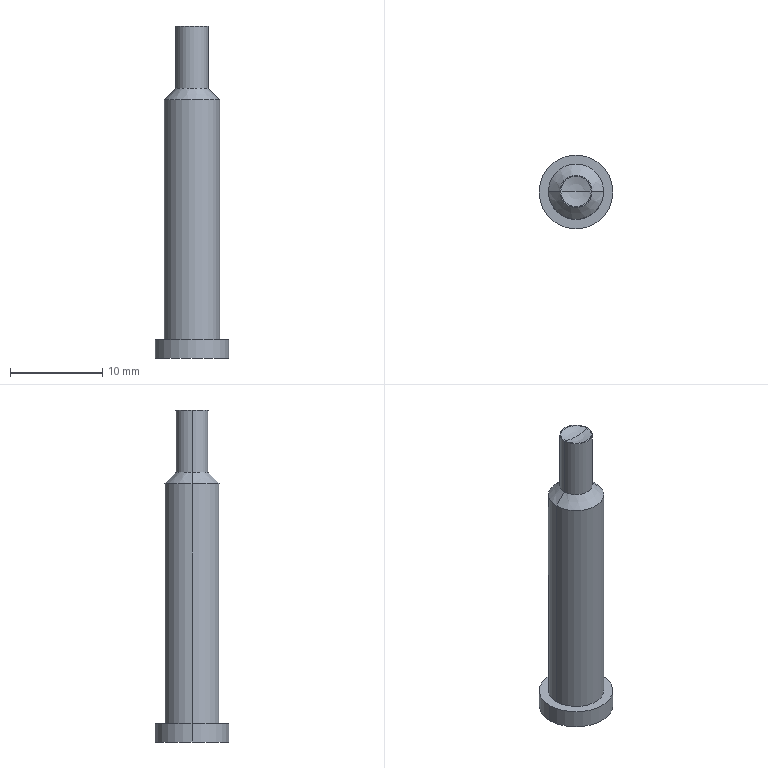Part | STEP file | Hot-melt nozzle | 1 solid | 13 faces | box 8 x 8 x 36 mm | volume 921.971 mm3 | cylinder 6 | plane 3 | cone 2 | sphere 2 | commonest cylinder face diameters 3.5 x2 6 x2 8 x2
STEP:
#1=CARTESIAN_POINT('',(0.,0.,0.));
#2=DIRECTION('',(0.,0.,1.));
#3=DIRECTION('',(1.,0.,0.));
#4=AXIS2_PLACEMENT_3D('',#1,#2,#3);
#5=CARTESIAN_POINT('',(139.55,-164.6,-40.7));
#6=VERTEX_POINT('',#5);
#7=CARTESIAN_POINT('',(147.55,-164.6,-40.7));
#8=VERTEX_POINT('',#7);
#9=CARTESIAN_POINT('',(143.55,-164.6,-40.7));
#10=DIRECTION('',(0.,0.,-1.));
#11=DIRECTION('',(-1.,0.,0.));
#12=AXIS2_PLACEMENT_3D('',#9,#10,#11);
#13=CIRCLE('',#12,4.);
#14=CARTESIAN_POINT('',(0.,0.,-40.7));
#15=DIRECTION('',(0.,0.,-1.));
#16=DIRECTION('',(-1.,0.,0.));
#17=AXIS2_PLACEMENT_3D('',#14,#15,#16);
#18=PLANE('',#17);
#19=CARTESIAN_POINT('',(-143.55,-164.6));
#20=DIRECTION('',(1.,0.));
#21=AXIS2_PLACEMENT_2D('',#19,#20);
#22=CIRCLE('',#21,4.);
#23=(GEOMETRIC_REPRESENTATION_CONTEXT(2)PARAMETRIC_REPRESENTATION_CONTEXT()REPRESENTATION_CONTEXT('',''));
#24=DEFINITIONAL_REPRESENTATION('',(#22),#23);
#25=PCURVE('',#18,#24);
#26=CARTESIAN_POINT('',(143.55,-164.6,-40.7));
#27=DIRECTION('',(0.,0.,-1.));
#28=DIRECTION('',(-1.,0.,0.));
#29=AXIS2_PLACEMENT_3D('',#26,#27,#28);
#30=CYLINDRICAL_SURFACE('',#29,4.);
#31=CARTESIAN_POINT('',(0.,0.));
#32=DIRECTION('',(1.,0.));
#33=VECTOR('',#32,1.);
#34=LINE('',#31,#33);
#35=(GEOMETRIC_REPRESENTATION_CONTEXT(2)PARAMETRIC_REPRESENTATION_CONTEXT()REPRESENTATION_CONTEXT('',''));
#36=DEFINITIONAL_REPRESENTATION('',(#34),#35);
#37=PCURVE('',#30,#36);
#38=SURFACE_CURVE('',#13,(#25,#37),.PCURVE_S1.);
#39=EDGE_CURVE('',#6,#8,#38,.T.);
#40=ORIENTED_EDGE('',*,*,#39,.F.);
#41=CARTESIAN_POINT('',(143.55,-164.6,-40.7));
#42=DIRECTION('',(0.,0.,-1.));
#43=DIRECTION('',(1.,0.,0.));
#44=AXIS2_PLACEMENT_3D('',#41,#42,#43);
#45=CIRCLE('',#44,4.);
#46=CARTESIAN_POINT('',(-143.55,-164.6));
#47=DIRECTION('',(-1.,0.));
#48=AXIS2_PLACEMENT_2D('',#46,#47);
#49=CIRCLE('',#48,4.);
#50=(GEOMETRIC_REPRESENTATION_CONTEXT(2)PARAMETRIC_REPRESENTATION_CONTEXT()REPRESENTATION_CONTEXT('',''));
#51=DEFINITIONAL_REPRESENTATION('',(#49),#50);
#52=PCURVE('',#18,#51);
#53=CARTESIAN_POINT('',(143.55,-164.6,-40.7));
#54=DIRECTION('',(0.,0.,-1.));
#55=DIRECTION('',(-1.,0.,0.));
#56=AXIS2_PLACEMENT_3D('',#53,#54,#55);
#57=CYLINDRICAL_SURFACE('',#56,4.);
#58=CARTESIAN_POINT('',(3.142,0.));
#59=DIRECTION('',(1.,0.));
#60=VECTOR('',#59,1.);
#61=LINE('',#58,#60);
#62=(GEOMETRIC_REPRESENTATION_CONTEXT(2)PARAMETRIC_REPRESENTATION_CONTEXT()REPRESENTATION_CONTEXT('',''));
#63=DEFINITIONAL_REPRESENTATION('',(#61),#62);
#64=PCURVE('',#57,#63);
#65=SURFACE_CURVE('',#45,(#52,#64),.PCURVE_S1.);
#66=EDGE_CURVE('',#8,#6,#65,.T.);
#67=ORIENTED_EDGE('',*,*,#66,.F.);
#68=EDGE_LOOP('',(#40,#67));
#69=FACE_BOUND('',#68,.F.);
#70=ADVANCED_FACE('',(#69),#18,.T.);
#71=CARTESIAN_POINT('',(139.55,-164.6,-38.7));
#72=VERTEX_POINT('',#71);
#73=CARTESIAN_POINT('',(139.55,-164.6,-40.7));
#74=DIRECTION('',(0.,0.,1.));
#75=VECTOR('',#74,1.);
#76=LINE('',#73,#75);
#77=CARTESIAN_POINT('',(0.,0.));
#78=DIRECTION('',(0.,-1.));
#79=VECTOR('',#78,1.);
#80=LINE('',#77,#79);
#81=(GEOMETRIC_REPRESENTATION_CONTEXT(2)PARAMETRIC_REPRESENTATION_CONTEXT()REPRESENTATION_CONTEXT('',''));
#82=DEFINITIONAL_REPRESENTATION('',(#80),#81);
#83=PCURVE('',#30,#82);
#84=CARTESIAN_POINT('',(6.283,0.));
#85=DIRECTION('',(0.,-1.));
#86=VECTOR('',#85,1.);
#87=LINE('',#84,#86);
#88=(GEOMETRIC_REPRESENTATION_CONTEXT(2)PARAMETRIC_REPRESENTATION_CONTEXT()REPRESENTATION_CONTEXT('',''));
#89=DEFINITIONAL_REPRESENTATION('',(#87),#88);
#90=PCURVE('',#57,#89);
#91=SURFACE_CURVE('',#76,(#83,#90),.PCURVE_S1.);
#92=EDGE_CURVE('',#6,#72,#91,.T.);
#93=ORIENTED_EDGE('',*,*,#92,.T.);
#94=CARTESIAN_POINT('',(147.55,-164.6,-38.7));
#95=VERTEX_POINT('',#94);
#96=CARTESIAN_POINT('',(143.55,-164.6,-38.7));
#97=DIRECTION('',(0.,0.,-1.));
#98=DIRECTION('',(-1.,0.,0.));
#99=AXIS2_PLACEMENT_3D('',#96,#97,#98);
#100=CIRCLE('',#99,4.);
#101=CARTESIAN_POINT('',(0.,-2.));
#102=DIRECTION('',(1.,0.));
#103=VECTOR('',#102,1.);
#104=LINE('',#101,#103);
#105=(GEOMETRIC_REPRESENTATION_CONTEXT(2)PARAMETRIC_REPRESENTATION_CONTEXT()REPRESENTATION_CONTEXT('',''));
#106=DEFINITIONAL_REPRESENTATION('',(#104),#105);
#107=PCURVE('',#30,#106);
#108=CARTESIAN_POINT('',(0.,0.,-38.7));
#109=DIRECTION('',(0.,0.,-1.));
#110=DIRECTION('',(-1.,0.,0.));
#111=AXIS2_PLACEMENT_3D('',#108,#109,#110);
#112=PLANE('',#111);
#113=CARTESIAN_POINT('',(-143.55,-164.6));
#114=DIRECTION('',(1.,0.));
#115=AXIS2_PLACEMENT_2D('',#113,#114);
#116=CIRCLE('',#115,4.);
#117=(GEOMETRIC_REPRESENTATION_CONTEXT(2)PARAMETRIC_REPRESENTATION_CONTEXT()REPRESENTATION_CONTEXT('',''));
#118=DEFINITIONAL_REPRESENTATION('',(#116),#117);
#119=PCURVE('',#112,#118);
#120=SURFACE_CURVE('',#100,(#107,#119),.PCURVE_S1.);
#121=EDGE_CURVE('',#72,#95,#120,.T.);
#122=ORIENTED_EDGE('',*,*,#121,.T.);
#123=CARTESIAN_POINT('',(147.55,-164.6,-40.7));
#124=DIRECTION('',(0.,0.,1.));
#125=VECTOR('',#124,1.);
#126=LINE('',#123,#125);
#127=CARTESIAN_POINT('',(3.142,0.));
#128=DIRECTION('',(0.,-1.));
#129=VECTOR('',#128,1.);
#130=LINE('',#127,#129);
#131=(GEOMETRIC_REPRESENTATION_CONTEXT(2)PARAMETRIC_REPRESENTATION_CONTEXT()REPRESENTATION_CONTEXT('',''));
#132=DEFINITIONAL_REPRESENTATION('',(#130),#131);
#133=PCURVE('',#30,#132);
#134=CARTESIAN_POINT('',(3.142,0.));
#135=DIRECTION('',(0.,-1.));
#136=VECTOR('',#135,1.);
#137=LINE('',#134,#136);
#138=(GEOMETRIC_REPRESENTATION_CONTEXT(2)PARAMETRIC_REPRESENTATION_CONTEXT()REPRESENTATION_CONTEXT('',''));
#139=DEFINITIONAL_REPRESENTATION('',(#137),#138);
#140=PCURVE('',#57,#139);
#141=SURFACE_CURVE('',#126,(#133,#140),.PCURVE_S1.);
#142=EDGE_CURVE('',#8,#95,#141,.T.);
#143=ORIENTED_EDGE('',*,*,#142,.F.);
#144=ORIENTED_EDGE('',*,*,#39,.F.);
#145=EDGE_LOOP('',(#93,#122,#143,#144));
#146=FACE_BOUND('',#145,.T.);
#147=ADVANCED_FACE('',(#146),#30,.T.);
#148=ORIENTED_EDGE('',*,*,#142,.T.);
#149=CARTESIAN_POINT('',(143.55,-164.6,-38.7));
#150=DIRECTION('',(0.,0.,-1.));
#151=DIRECTION('',(1.,0.,0.));
#152=AXIS2_PLACEMENT_3D('',#149,#150,#151);
#153=CIRCLE('',#152,4.);
#154=CARTESIAN_POINT('',(3.142,-2.));
#155=DIRECTION('',(1.,0.));
#156=VECTOR('',#155,1.);
#157=LINE('',#154,#156);
#158=(GEOMETRIC_REPRESENTATION_CONTEXT(2)PARAMETRIC_REPRESENTATION_CONTEXT()REPRESENTATION_CONTEXT('',''));
#159=DEFINITIONAL_REPRESENTATION('',(#157),#158);
#160=PCURVE('',#57,#159);
#161=CARTESIAN_POINT('',(-143.55,-164.6));
#162=DIRECTION('',(-1.,0.));
#163=AXIS2_PLACEMENT_2D('',#161,#162);
#164=CIRCLE('',#163,4.);
#165=(GEOMETRIC_REPRESENTATION_CONTEXT(2)PARAMETRIC_REPRESENTATION_CONTEXT()REPRESENTATION_CONTEXT('',''));
#166=DEFINITIONAL_REPRESENTATION('',(#164),#165);
#167=PCURVE('',#112,#166);
#168=SURFACE_CURVE('',#153,(#160,#167),.PCURVE_S1.);
#169=EDGE_CURVE('',#95,#72,#168,.T.);
#170=ORIENTED_EDGE('',*,*,#169,.T.);
#171=ORIENTED_EDGE('',*,*,#92,.F.);
#172=ORIENTED_EDGE('',*,*,#66,.F.);
#173=EDGE_LOOP('',(#148,#170,#171,#172));
#174=FACE_BOUND('',#173,.T.);
#175=ADVANCED_FACE('',(#174),#57,.T.);
#176=ORIENTED_EDGE('',*,*,#121,.T.);
#177=ORIENTED_EDGE('',*,*,#169,.T.);
#178=EDGE_LOOP('',(#176,#177));
#179=FACE_BOUND('',#178,.F.);
#180=CARTESIAN_POINT('',(140.55,-164.6,-38.7));
#181=VERTEX_POINT('',#180);
#182=CARTESIAN_POINT('',(146.55,-164.6,-38.7));
#183=VERTEX_POINT('',#182);
#184=CARTESIAN_POINT('',(143.55,-164.6,-38.7));
#185=DIRECTION('',(0.,0.,-1.));
#186=DIRECTION('',(-1.,0.,0.));
#187=AXIS2_PLACEMENT_3D('',#184,#185,#186);
#188=CIRCLE('',#187,3.);
#189=CARTESIAN_POINT('',(-143.55,-164.6));
#190=DIRECTION('',(1.,0.));
#191=AXIS2_PLACEMENT_2D('',#189,#190);
#192=CIRCLE('',#191,3.);
#193=(GEOMETRIC_REPRESENTATION_CONTEXT(2)PARAMETRIC_REPRESENTATION_CONTEXT()REPRESENTATION_CONTEXT('',''));
#194=DEFINITIONAL_REPRESENTATION('',(#192),#193);
#195=PCURVE('',#112,#194);
#196=CARTESIAN_POINT('',(143.55,-164.6,-40.7));
#197=DIRECTION('',(0.,0.,-1.));
#198=DIRECTION('',(-1.,0.,0.));
#199=AXIS2_PLACEMENT_3D('',#196,#197,#198);
#200=CYLINDRICAL_SURFACE('',#199,3.);
#201=CARTESIAN_POINT('',(0.,-2.));
#202=DIRECTION('',(1.,0.));
#203=VECTOR('',#202,1.);
#204=LINE('',#201,#203);
#205=(GEOMETRIC_REPRESENTATION_CONTEXT(2)PARAMETRIC_REPRESENTATION_CONTEXT()REPRESENTATION_CONTEXT('',''));
#206=DEFINITIONAL_REPRESENTATION('',(#204),#205);
#207=PCURVE('',#200,#206);
#208=SURFACE_CURVE('',#188,(#195,#207),.PCURVE_S1.);
#209=EDGE_CURVE('',#181,#183,#208,.T.);
#210=ORIENTED_EDGE('',*,*,#209,.F.);
#211=CARTESIAN_POINT('',(143.55,-164.6,-38.7));
#212=DIRECTION('',(0.,0.,-1.));
#213=DIRECTION('',(1.,0.,0.));
#214=AXIS2_PLACEMENT_3D('',#211,#212,#213);
#215=CIRCLE('',#214,3.);
#216=CARTESIAN_POINT('',(-143.55,-164.6));
#217=DIRECTION('',(-1.,0.));
#218=AXIS2_PLACEMENT_2D('',#216,#217);
#219=CIRCLE('',#218,3.);
#220=(GEOMETRIC_REPRESENTATION_CONTEXT(2)PARAMETRIC_REPRESENTATION_CONTEXT()REPRESENTATION_CONTEXT('',''));
#221=DEFINITIONAL_REPRESENTATION('',(#219),#220);
#222=PCURVE('',#112,#221);
#223=CARTESIAN_POINT('',(143.55,-164.6,-40.7));
#224=DIRECTION('',(0.,0.,-1.));
#225=DIRECTION('',(-1.,0.,0.));
#226=AXIS2_PLACEMENT_3D('',#223,#224,#225);
#227=CYLINDRICAL_SURFACE('',#226,3.);
#228=CARTESIAN_POINT('',(3.142,-2.));
#229=DIRECTION('',(1.,0.));
#230=VECTOR('',#229,1.);
#231=LINE('',#228,#230);
#232=(GEOMETRIC_REPRESENTATION_CONTEXT(2)PARAMETRIC_REPRESENTATION_CONTEXT()REPRESENTATION_CONTEXT('',''));
#233=DEFINITIONAL_REPRESENTATION('',(#231),#232);
#234=PCURVE('',#227,#233);
#235=SURFACE_CURVE('',#215,(#222,#234),.PCURVE_S1.);
#236=EDGE_CURVE('',#183,#181,#235,.T.);
#237=ORIENTED_EDGE('',*,*,#236,.F.);
#238=EDGE_LOOP('',(#210,#237));
#239=FACE_BOUND('',#238,.F.);
#240=ADVANCED_FACE('',(#179,#239),#112,.F.);
#241=CARTESIAN_POINT('',(146.55,-164.6,-12.7));
#242=VERTEX_POINT('',#241);
#243=CARTESIAN_POINT('',(146.55,-164.6,-38.7));
#244=DIRECTION('',(-0.000000097,0.,1.));
#245=VECTOR('',#244,1.);
#246=LINE('',#243,#245);
#247=CARTESIAN_POINT('',(3.142,-2.));
#248=DIRECTION('',(0.,-1.));
#249=VECTOR('',#248,1.);
#250=LINE('',#247,#249);
#251=(GEOMETRIC_REPRESENTATION_CONTEXT(2)PARAMETRIC_REPRESENTATION_CONTEXT()REPRESENTATION_CONTEXT('',''));
#252=DEFINITIONAL_REPRESENTATION('',(#250),#251);
#253=PCURVE('',#200,#252);
#254=CARTESIAN_POINT('',(3.142,-2.));
#255=DIRECTION('',(0.,-1.));
#256=VECTOR('',#255,1.);
#257=LINE('',#254,#256);
#258=(GEOMETRIC_REPRESENTATION_CONTEXT(2)PARAMETRIC_REPRESENTATION_CONTEXT()REPRESENTATION_CONTEXT('',''));
#259=DEFINITIONAL_REPRESENTATION('',(#257),#258);
#260=PCURVE('',#227,#259);
#261=SURFACE_CURVE('',#246,(#253,#260),.PCURVE_S1.);
#262=EDGE_CURVE('',#183,#242,#261,.T.);
#263=ORIENTED_EDGE('',*,*,#262,.F.);
#264=ORIENTED_EDGE('',*,*,#209,.F.);
#265=CARTESIAN_POINT('',(140.55,-164.6,-12.7));
#266=VERTEX_POINT('',#265);
#267=CARTESIAN_POINT('',(140.55,-164.6,-38.7));
#268=DIRECTION('',(0.000000097,0.,1.));
#269=VECTOR('',#268,1.);
#270=LINE('',#267,#269);
#271=CARTESIAN_POINT('',(0.,-2.));
#272=DIRECTION('',(0.,-1.));
#273=VECTOR('',#272,1.);
#274=LINE('',#271,#273);
#275=(GEOMETRIC_REPRESENTATION_CONTEXT(2)PARAMETRIC_REPRESENTATION_CONTEXT()REPRESENTATION_CONTEXT('',''));
#276=DEFINITIONAL_REPRESENTATION('',(#274),#275);
#277=PCURVE('',#200,#276);
#278=CARTESIAN_POINT('',(6.283,-2.));
#279=DIRECTION('',(0.,-1.));
#280=VECTOR('',#279,1.);
#281=LINE('',#278,#280);
#282=(GEOMETRIC_REPRESENTATION_CONTEXT(2)PARAMETRIC_REPRESENTATION_CONTEXT()REPRESENTATION_CONTEXT('',''));
#283=DEFINITIONAL_REPRESENTATION('',(#281),#282);
#284=PCURVE('',#227,#283);
#285=SURFACE_CURVE('',#270,(#277,#284),.PCURVE_S1.);
#286=EDGE_CURVE('',#181,#266,#285,.T.);
#287=ORIENTED_EDGE('',*,*,#286,.T.);
#288=CARTESIAN_POINT('',(143.55,-164.6,-12.7));
#289=DIRECTION('',(0.,0.,1.));
#290=DIRECTION('',(1.,0.,0.));
#291=AXIS2_PLACEMENT_3D('',#288,#289,#290);
#292=CIRCLE('',#291,3.);
#293=CARTESIAN_POINT('',(3.142,-28.));
#294=DIRECTION('',(-1.,0.));
#295=VECTOR('',#294,1.);
#296=LINE('',#293,#295);
#297=(GEOMETRIC_REPRESENTATION_CONTEXT(2)PARAMETRIC_REPRESENTATION_CONTEXT()REPRESENTATION_CONTEXT('',''));
#298=DEFINITIONAL_REPRESENTATION('',(#296),#297);
#299=PCURVE('',#200,#298);
#300=CARTESIAN_POINT('',(143.55,-164.6,-12.075));
#301=DIRECTION('',(0.,0.,-1.));
#302=DIRECTION('',(0.,-1.,0.));
#303=AXIS2_PLACEMENT_3D('',#300,#301,#302);
#304=CONICAL_SURFACE('',#303,2.375,0.7854);
#305=CARTESIAN_POINT('',(4.712,0.625));
#306=DIRECTION('',(-1.,0.));
#307=VECTOR('',#306,1.);
#308=LINE('',#305,#307);
#309=(GEOMETRIC_REPRESENTATION_CONTEXT(2)PARAMETRIC_REPRESENTATION_CONTEXT()REPRESENTATION_CONTEXT('',''));
#310=DEFINITIONAL_REPRESENTATION('',(#308),#309);
#311=PCURVE('',#304,#310);
#312=SURFACE_CURVE('',#292,(#299,#311),.PCURVE_S1.);
#313=EDGE_CURVE('',#242,#266,#312,.T.);
#314=ORIENTED_EDGE('',*,*,#313,.F.);
#315=EDGE_LOOP('',(#263,#264,#287,#314));
#316=FACE_BOUND('',#315,.T.);
#317=ADVANCED_FACE('',(#316),#200,.T.);
#318=CARTESIAN_POINT('',(141.8,-164.6,-11.45));
#319=VERTEX_POINT('',#318);
#320=CARTESIAN_POINT('',(140.55,-164.6,-12.7));
#321=DIRECTION('',(0.7071,-0.000000001,0.7071));
#322=VECTOR('',#321,1.);
#323=LINE('',#320,#322);
#324=CARTESIAN_POINT('',(1.571,0.625));
#325=DIRECTION('',(0.,-1.));
#326=VECTOR('',#325,1.);
#327=LINE('',#324,#326);
#328=(GEOMETRIC_REPRESENTATION_CONTEXT(2)PARAMETRIC_REPRESENTATION_CONTEXT()REPRESENTATION_CONTEXT('',''));
#329=DEFINITIONAL_REPRESENTATION('',(#327),#328);
#330=PCURVE('',#304,#329);
#331=CARTESIAN_POINT('',(143.55,-164.6,-12.075));
#332=DIRECTION('',(0.,0.,-1.));
#333=DIRECTION('',(0.,-1.,0.));
#334=AXIS2_PLACEMENT_3D('',#331,#332,#333);
#335=CONICAL_SURFACE('',#334,2.375,0.7854);
#336=CARTESIAN_POINT('',(1.571,0.625));
#337=DIRECTION('',(0.,-1.));
#338=VECTOR('',#337,1.);
#339=LINE('',#336,#338);
#340=(GEOMETRIC_REPRESENTATION_CONTEXT(2)PARAMETRIC_REPRESENTATION_CONTEXT()REPRESENTATION_CONTEXT('',''));
#341=DEFINITIONAL_REPRESENTATION('',(#339),#340);
#342=PCURVE('',#335,#341);
#343=SURFACE_CURVE('',#323,(#330,#342),.PCURVE_S1.);
#344=EDGE_CURVE('',#266,#319,#343,.T.);
#345=ORIENTED_EDGE('',*,*,#344,.T.);
#346=CARTESIAN_POINT('',(145.3,-164.6,-11.45));
#347=VERTEX_POINT('',#346);
#348=CARTESIAN_POINT('',(143.55,-164.6,-11.45));
#349=DIRECTION('',(0.,0.,1.));
#350=DIRECTION('',(1.,0.,0.));
#351=AXIS2_PLACEMENT_3D('',#348,#349,#350);
#352=CIRCLE('',#351,1.75);
#353=CARTESIAN_POINT('',(4.712,-0.625));
#354=DIRECTION('',(-1.,0.));
#355=VECTOR('',#354,1.);
#356=LINE('',#353,#355);
#357=(GEOMETRIC_REPRESENTATION_CONTEXT(2)PARAMETRIC_REPRESENTATION_CONTEXT()REPRESENTATION_CONTEXT('',''));
#358=DEFINITIONAL_REPRESENTATION('',(#356),#357);
#359=PCURVE('',#304,#358);
#360=CARTESIAN_POINT('',(143.55,-164.6,-4.7));
#361=DIRECTION('',(0.,0.,1.));
#362=DIRECTION('',(1.,0.,0.));
#363=AXIS2_PLACEMENT_3D('',#360,#361,#362);
#364=CYLINDRICAL_SURFACE('',#363,1.75);
#365=CARTESIAN_POINT('',(0.,-6.75));
#366=DIRECTION('',(1.,0.));
#367=VECTOR('',#366,1.);
#368=LINE('',#365,#367);
#369=(GEOMETRIC_REPRESENTATION_CONTEXT(2)PARAMETRIC_REPRESENTATION_CONTEXT()REPRESENTATION_CONTEXT('',''));
#370=DEFINITIONAL_REPRESENTATION('',(#368),#369);
#371=PCURVE('',#364,#370);
#372=SURFACE_CURVE('',#352,(#359,#371),.PCURVE_S1.);
#373=EDGE_CURVE('',#347,#319,#372,.T.);
#374=ORIENTED_EDGE('',*,*,#373,.F.);
#375=CARTESIAN_POINT('',(146.55,-164.6,-12.7));
#376=DIRECTION('',(-0.7071,0.000000001,0.7071));
#377=VECTOR('',#376,1.);
#378=LINE('',#375,#377);
#379=CARTESIAN_POINT('',(4.712,0.625));
#380=DIRECTION('',(0.,-1.));
#381=VECTOR('',#380,1.);
#382=LINE('',#379,#381);
#383=(GEOMETRIC_REPRESENTATION_CONTEXT(2)PARAMETRIC_REPRESENTATION_CONTEXT()REPRESENTATION_CONTEXT('',''));
#384=DEFINITIONAL_REPRESENTATION('',(#382),#383);
#385=PCURVE('',#304,#384);
#386=CARTESIAN_POINT('',(-1.571,0.625));
#387=DIRECTION('',(0.,-1.));
#388=VECTOR('',#387,1.);
#389=LINE('',#386,#388);
#390=(GEOMETRIC_REPRESENTATION_CONTEXT(2)PARAMETRIC_REPRESENTATION_CONTEXT()REPRESENTATION_CONTEXT('',''));
#391=DEFINITIONAL_REPRESENTATION('',(#389),#390);
#392=PCURVE('',#335,#391);
#393=SURFACE_CURVE('',#378,(#385,#392),.PCURVE_S1.);
#394=EDGE_CURVE('',#242,#347,#393,.T.);
#395=ORIENTED_EDGE('',*,*,#394,.F.);
#396=ORIENTED_EDGE('',*,*,#313,.T.);
#397=EDGE_LOOP('',(#345,#374,#395,#396));
#398=FACE_BOUND('',#397,.T.);
#399=ADVANCED_FACE('',(#398),#304,.T.);
#400=ORIENTED_EDGE('',*,*,#394,.T.);
#401=CARTESIAN_POINT('',(143.55,-164.6,-11.45));
#402=DIRECTION('',(0.,0.,1.));
#403=DIRECTION('',(-1.,0.,0.));
#404=AXIS2_PLACEMENT_3D('',#401,#402,#403);
#405=CIRCLE('',#404,1.75);
#406=CARTESIAN_POINT('',(1.571,-0.625));
#407=DIRECTION('',(-1.,0.));
#408=VECTOR('',#407,1.);
#409=LINE('',#406,#408);
#410=(GEOMETRIC_REPRESENTATION_CONTEXT(2)PARAMETRIC_REPRESENTATION_CONTEXT()REPRESENTATION_CONTEXT('',''));
#411=DEFINITIONAL_REPRESENTATION('',(#409),#410);
#412=PCURVE('',#335,#411);
#413=CARTESIAN_POINT('',(143.55,-164.6,-4.7));
#414=DIRECTION('',(0.,0.,1.));
#415=DIRECTION('',(1.,0.,0.));
#416=AXIS2_PLACEMENT_3D('',#413,#414,#415);
#417=CYLINDRICAL_SURFACE('',#416,1.75);
#418=CARTESIAN_POINT('',(3.142,-6.75));
#419=DIRECTION('',(1.,0.));
#420=VECTOR('',#419,1.);
#421=LINE('',#418,#420);
#422=(GEOMETRIC_REPRESENTATION_CONTEXT(2)PARAMETRIC_REPRESENTATION_CONTEXT()REPRESENTATION_CONTEXT('',''));
#423=DEFINITIONAL_REPRESENTATION('',(#421),#422);
#424=PCURVE('',#417,#423);
#425=SURFACE_CURVE('',#405,(#412,#424),.PCURVE_S1.);
#426=EDGE_CURVE('',#319,#347,#425,.T.);
#427=ORIENTED_EDGE('',*,*,#426,.F.);
#428=ORIENTED_EDGE('',*,*,#344,.F.);
#429=CARTESIAN_POINT('',(143.55,-164.6,-12.7));
#430=DIRECTION('',(0.,0.,1.));
#431=DIRECTION('',(-1.,0.,0.));
#432=AXIS2_PLACEMENT_3D('',#429,#430,#431);
#433=CIRCLE('',#432,3.);
#434=CARTESIAN_POINT('',(1.571,0.625));
#435=DIRECTION('',(-1.,0.));
#436=VECTOR('',#435,1.);
#437=LINE('',#434,#436);
#438=(GEOMETRIC_REPRESENTATION_CONTEXT(2)PARAMETRIC_REPRESENTATION_CONTEXT()REPRESENTATION_CONTEXT('',''));
#439=DEFINITIONAL_REPRESENTATION('',(#437),#438);
#440=PCURVE('',#335,#439);
#441=CARTESIAN_POINT('',(6.283,-28.));
#442=DIRECTION('',(-1.,0.));
#443=VECTOR('',#442,1.);
#444=LINE('',#441,#443);
#445=(GEOMETRIC_REPRESENTATION_CONTEXT(2)PARAMETRIC_REPRESENTATION_CONTEXT()REPRESENTATION_CONTEXT('',''));
#446=DEFINITIONAL_REPRESENTATION('',(#444),#445);
#447=PCURVE('',#227,#446);
#448=SURFACE_CURVE('',#433,(#440,#447),.PCURVE_S1.);
#449=EDGE_CURVE('',#266,#242,#448,.T.);
#450=ORIENTED_EDGE('',*,*,#449,.T.);
#451=EDGE_LOOP('',(#400,#427,#428,#450));
#452=FACE_BOUND('',#451,.T.);
#453=ADVANCED_FACE('',(#452),#335,.T.);
#454=ORIENTED_EDGE('',*,*,#286,.F.);
#455=ORIENTED_EDGE('',*,*,#236,.F.);
#456=ORIENTED_EDGE('',*,*,#262,.T.);
#457=ORIENTED_EDGE('',*,*,#449,.F.);
#458=EDGE_LOOP('',(#454,#455,#456,#457));
#459=FACE_BOUND('',#458,.T.);
#460=ADVANCED_FACE('',(#459),#227,.T.);
#461=CARTESIAN_POINT('',(145.3,-164.6,-4.7));
#462=VERTEX_POINT('',#461);
#463=CARTESIAN_POINT('',(145.3,-164.6,-4.7));
#464=DIRECTION('',(-0.000000218,-0.000000001,-1.));
#465=VECTOR('',#464,1.);
#466=LINE('',#463,#465);
#467=CARTESIAN_POINT('',(6.283,0.));
#468=CARTESIAN_POINT('',(6.283,-0.1023));
#469=CARTESIAN_POINT('',(6.283,-0.3068));
#470=CARTESIAN_POINT('',(6.283,-0.6136));
#471=CARTESIAN_POINT('',(6.283,-0.9205));
#472=CARTESIAN_POINT('',(6.283,-1.227));
#473=CARTESIAN_POINT('',(6.283,-1.534));
#474=CARTESIAN_POINT('',(6.283,-1.841));
#475=CARTESIAN_POINT('',(6.283,-2.148));
#476=CARTESIAN_POINT('',(6.283,-2.455));
#477=CARTESIAN_POINT('',(6.283,-2.761));
#478=CARTESIAN_POINT('',(6.283,-3.068));
#479=CARTESIAN_POINT('',(6.283,-3.375));
#480=CARTESIAN_POINT('',(6.283,-3.682));
#481=CARTESIAN_POINT('',(6.283,-3.989));
#482=CARTESIAN_POINT('',(6.283,-4.295));
#483=CARTESIAN_POINT('',(6.283,-4.602));
#484=CARTESIAN_POINT('',(6.283,-4.909));
#485=CARTESIAN_POINT('',(6.283,-5.216));
#486=CARTESIAN_POINT('',(6.283,-5.523));
#487=CARTESIAN_POINT('',(6.283,-5.83));
#488=CARTESIAN_POINT('',(6.283,-6.136));
#489=CARTESIAN_POINT('',(6.283,-6.443));
#490=CARTESIAN_POINT('',(6.283,-6.648));
#491=CARTESIAN_POINT('',(6.283,-6.75));
#492=B_SPLINE_CURVE_WITH_KNOTS('',3,(#467,#468,#469,#470,#471,#472,#473,#474,#475,#476,#477,#478,#479,#480,#481,#482,#483,#484,#485,#486,#487,#488,#489,#490,#491),.UNSPECIFIED.,.F.,.F.,(4,1,1,1,1,1,1,1,1,1,1,1,1,1,1,1,1,1,1,1,1,1,4),(0.,0.3068,0.6136,0.9205,1.227,1.534,1.841,2.148,2.455,2.761,3.068,3.375,3.682,3.989,4.295,4.602,4.909,5.216,5.523,5.83,6.136,6.443,6.75),.QUASI_UNIFORM_KNOTS.);
#493=(GEOMETRIC_REPRESENTATION_CONTEXT(2)PARAMETRIC_REPRESENTATION_CONTEXT()REPRESENTATION_CONTEXT('',''));
#494=DEFINITIONAL_REPRESENTATION('',(#492),#493);
#495=PCURVE('',#417,#494);
#496=CARTESIAN_POINT('',(0.,0.));
#497=CARTESIAN_POINT('',(0.,-0.1023));
#498=CARTESIAN_POINT('',(0.,-0.3068));
#499=CARTESIAN_POINT('',(0.,-0.6136));
#500=CARTESIAN_POINT('',(0.,-0.9205));
#501=CARTESIAN_POINT('',(0.,-1.227));
#502=CARTESIAN_POINT('',(0.,-1.534));
#503=CARTESIAN_POINT('',(-0.000000001,-1.841));
#504=CARTESIAN_POINT('',(-0.000000001,-2.148));
#505=CARTESIAN_POINT('',(-0.000000001,-2.455));
#506=CARTESIAN_POINT('',(-0.000000001,-2.761));
#507=CARTESIAN_POINT('',(-0.000000001,-3.068));
#508=CARTESIAN_POINT('',(-0.000000001,-3.375));
#509=CARTESIAN_POINT('',(-0.000000001,-3.682));
#510=CARTESIAN_POINT('',(-0.000000001,-3.989));
#511=CARTESIAN_POINT('',(-0.000000001,-4.295));
#512=CARTESIAN_POINT('',(-0.000000001,-4.602));
#513=CARTESIAN_POINT('',(-0.000000002,-4.909));
#514=CARTESIAN_POINT('',(-0.000000002,-5.216));
#515=CARTESIAN_POINT('',(-0.000000002,-5.523));
#516=CARTESIAN_POINT('',(-0.000000002,-5.83));
#517=CARTESIAN_POINT('',(-0.000000002,-6.136));
#518=CARTESIAN_POINT('',(-0.000000002,-6.443));
#519=CARTESIAN_POINT('',(-0.000000002,-6.648));
#520=CARTESIAN_POINT('',(-0.000000002,-6.75));
#521=B_SPLINE_CURVE_WITH_KNOTS('',3,(#496,#497,#498,#499,#500,#501,#502,#503,#504,#505,#506,#507,#508,#509,#510,#511,#512,#513,#514,#515,#516,#517,#518,#519,#520),.UNSPECIFIED.,.F.,.F.,(4,1,1,1,1,1,1,1,1,1,1,1,1,1,1,1,1,1,1,1,1,1,4),(0.,0.3068,0.6136,0.9205,1.227,1.534,1.841,2.148,2.455,2.761,3.068,3.375,3.682,3.989,4.295,4.602,4.909,5.216,5.523,5.83,6.136,6.443,6.75),.QUASI_UNIFORM_KNOTS.);
#522=(GEOMETRIC_REPRESENTATION_CONTEXT(2)PARAMETRIC_REPRESENTATION_CONTEXT()REPRESENTATION_CONTEXT('',''));
#523=DEFINITIONAL_REPRESENTATION('',(#521),#522);
#524=PCURVE('',#364,#523);
#525=SURFACE_CURVE('',#466,(#495,#524),.PCURVE_S1.);
#526=EDGE_CURVE('',#462,#347,#525,.T.);
#527=ORIENTED_EDGE('',*,*,#526,.F.);
#528=CARTESIAN_POINT('',(141.8,-164.6,-4.7));
#529=VERTEX_POINT('',#528);
#530=CARTESIAN_POINT('',(143.55,-164.6,-4.7));
#531=DIRECTION('',(0.,0.,1.));
#532=DIRECTION('',(-1.,0.,0.));
#533=AXIS2_PLACEMENT_3D('',#530,#531,#532);
#534=CIRCLE('',#533,1.75);
#535=CARTESIAN_POINT('',(3.142,0.));
#536=DIRECTION('',(1.,0.));
#537=VECTOR('',#536,1.);
#538=LINE('',#535,#537);
#539=(GEOMETRIC_REPRESENTATION_CONTEXT(2)PARAMETRIC_REPRESENTATION_CONTEXT()REPRESENTATION_CONTEXT('',''));
#540=DEFINITIONAL_REPRESENTATION('',(#538),#539);
#541=PCURVE('',#417,#540);
#542=CARTESIAN_POINT('',(0.,0.,-4.7));
#543=DIRECTION('',(0.,0.,-1.));
#544=DIRECTION('',(-1.,0.,0.));
#545=AXIS2_PLACEMENT_3D('',#542,#543,#544);
#546=PLANE('',#545);
#547=CARTESIAN_POINT('',(-141.8,-164.6));
#548=CARTESIAN_POINT('',(-141.8,-167.631));
#549=CARTESIAN_POINT('',(-144.425,-166.116));
#550=CARTESIAN_POINT('',(-147.05,-164.6));
#551=CARTESIAN_POINT('',(-144.425,-163.085));
#552=CARTESIAN_POINT('',(-141.8,-161.569));
#553=CARTESIAN_POINT('',(-141.8,-164.6));
#554=(BOUNDED_CURVE()B_SPLINE_CURVE(2,(#547,#548,#549,#550,#551,#552,#553),.UNSPECIFIED.,.T.,.F.)B_SPLINE_CURVE_WITH_KNOTS((1,2,2,2,2,1),(-2.094,0.,2.094,4.189,6.283,8.378),.UNSPECIFIED.)CURVE()GEOMETRIC_REPRESENTATION_ITEM()RATIONAL_B_SPLINE_CURVE((1.,0.5,1.,0.5,1.,0.5,1.))REPRESENTATION_ITEM(''));
#555=(GEOMETRIC_REPRESENTATION_CONTEXT(2)PARAMETRIC_REPRESENTATION_CONTEXT()REPRESENTATION_CONTEXT('',''));
#556=DEFINITIONAL_REPRESENTATION('',(#554),#555);
#557=PCURVE('',#546,#556);
#558=SURFACE_CURVE('',#534,(#541,#557),.PCURVE_S1.);
#559=EDGE_CURVE('',#529,#462,#558,.T.);
#560=ORIENTED_EDGE('',*,*,#559,.F.);
#561=CARTESIAN_POINT('',(141.8,-164.6,-4.7));
#562=DIRECTION('',(0.000000218,0.000000001,-1.));
#563=VECTOR('',#562,1.);
#564=LINE('',#561,#563);
#565=CARTESIAN_POINT('',(3.142,0.));
#566=DIRECTION('',(0.,-1.));
#567=VECTOR('',#566,1.);
#568=LINE('',#565,#567);
#569=(GEOMETRIC_REPRESENTATION_CONTEXT(2)PARAMETRIC_REPRESENTATION_CONTEXT()REPRESENTATION_CONTEXT('',''));
#570=DEFINITIONAL_REPRESENTATION('',(#568),#569);
#571=PCURVE('',#417,#570);
#572=CARTESIAN_POINT('',(3.142,0.));
#573=DIRECTION('',(0.,-1.));
#574=VECTOR('',#573,1.);
#575=LINE('',#572,#574);
#576=(GEOMETRIC_REPRESENTATION_CONTEXT(2)PARAMETRIC_REPRESENTATION_CONTEXT()REPRESENTATION_CONTEXT('',''));
#577=DEFINITIONAL_REPRESENTATION('',(#575),#576);
#578=PCURVE('',#364,#577);
#579=SURFACE_CURVE('',#564,(#571,#578),.PCURVE_S1.);
#580=EDGE_CURVE('',#529,#319,#579,.T.);
#581=ORIENTED_EDGE('',*,*,#580,.T.);
#582=ORIENTED_EDGE('',*,*,#426,.T.);
#583=EDGE_LOOP('',(#527,#560,#581,#582));
#584=FACE_BOUND('',#583,.T.);
#585=ADVANCED_FACE('',(#584),#417,.T.);
#586=ORIENTED_EDGE('',*,*,#580,.F.);
#587=CARTESIAN_POINT('',(143.55,-164.6,-4.7));
#588=DIRECTION('',(0.,0.,1.));
#589=DIRECTION('',(1.,0.,0.));
#590=AXIS2_PLACEMENT_3D('',#587,#588,#589);
#591=CIRCLE('',#590,1.75);
#592=CARTESIAN_POINT('',(0.,0.));
#593=DIRECTION('',(1.,0.));
#594=VECTOR('',#593,1.);
#595=LINE('',#592,#594);
#596=(GEOMETRIC_REPRESENTATION_CONTEXT(2)PARAMETRIC_REPRESENTATION_CONTEXT()REPRESENTATION_CONTEXT('',''));
#597=DEFINITIONAL_REPRESENTATION('',(#595),#596);
#598=PCURVE('',#364,#597);
#599=CARTESIAN_POINT('',(-145.3,-164.6));
#600=CARTESIAN_POINT('',(-145.3,-161.569));
#601=CARTESIAN_POINT('',(-142.675,-163.085));
#602=CARTESIAN_POINT('',(-140.05,-164.6));
#603=CARTESIAN_POINT('',(-142.675,-166.116));
#604=CARTESIAN_POINT('',(-145.3,-167.631));
#605=CARTESIAN_POINT('',(-145.3,-164.6));
#606=(BOUNDED_CURVE()B_SPLINE_CURVE(2,(#599,#600,#601,#602,#603,#604,#605),.UNSPECIFIED.,.T.,.F.)B_SPLINE_CURVE_WITH_KNOTS((1,2,2,2,2,1),(-2.094,0.,2.094,4.189,6.283,8.378),.UNSPECIFIED.)CURVE()GEOMETRIC_REPRESENTATION_ITEM()RATIONAL_B_SPLINE_CURVE((1.,0.5,1.,0.5,1.,0.5,1.))REPRESENTATION_ITEM(''));
#607=(GEOMETRIC_REPRESENTATION_CONTEXT(2)PARAMETRIC_REPRESENTATION_CONTEXT()REPRESENTATION_CONTEXT('',''));
#608=DEFINITIONAL_REPRESENTATION('',(#606),#607);
#609=PCURVE('',#546,#608);
#610=SURFACE_CURVE('',#591,(#598,#609),.PCURVE_S1.);
#611=EDGE_CURVE('',#462,#529,#610,.T.);
#612=ORIENTED_EDGE('',*,*,#611,.F.);
#613=ORIENTED_EDGE('',*,*,#526,.T.);
#614=ORIENTED_EDGE('',*,*,#373,.T.);
#615=EDGE_LOOP('',(#586,#612,#613,#614));
#616=FACE_BOUND('',#615,.T.);
#617=ADVANCED_FACE('',(#616),#364,.T.);
#618=ORIENTED_EDGE('',*,*,#559,.F.);
#619=ORIENTED_EDGE('',*,*,#611,.F.);
#620=EDGE_LOOP('',(#618,#619));
#621=FACE_BOUND('',#620,.F.);
#622=CARTESIAN_POINT('',(141.9,-164.6,-4.7));
#623=VERTEX_POINT('',#622);
#624=CARTESIAN_POINT('',(145.2,-164.6,-4.7));
#625=VERTEX_POINT('',#624);
#626=CARTESIAN_POINT('',(143.55,-164.6,-4.7));
#627=DIRECTION('',(0.,0.,-1.));
#628=DIRECTION('',(-1.,0.,0.));
#629=AXIS2_PLACEMENT_3D('',#626,#627,#628);
#630=CIRCLE('',#629,1.65);
#631=CARTESIAN_POINT('',(-143.55,-164.6));
#632=DIRECTION('',(1.,0.));
#633=AXIS2_PLACEMENT_2D('',#631,#632);
#634=CIRCLE('',#633,1.65);
#635=(GEOMETRIC_REPRESENTATION_CONTEXT(2)PARAMETRIC_REPRESENTATION_CONTEXT()REPRESENTATION_CONTEXT('',''));
#636=DEFINITIONAL_REPRESENTATION('',(#634),#635);
#637=PCURVE('',#546,#636);
#638=CARTESIAN_POINT('',(143.55,-164.6,-0.3125));
#639=DIRECTION('',(0.,0.,-1.));
#640=DIRECTION('',(1.,0.,0.));
#641=AXIS2_PLACEMENT_3D('',#638,#639,#640);
#642=SPHERICAL_SURFACE('',#641,4.688);
#643=CARTESIAN_POINT('',(3.142,1.211));
#644=CARTESIAN_POINT('',(3.189,1.211));
#645=CARTESIAN_POINT('',(3.284,1.211));
#646=CARTESIAN_POINT('',(3.427,1.211));
#647=CARTESIAN_POINT('',(3.57,1.211));
#648=CARTESIAN_POINT('',(3.713,1.211));
#649=CARTESIAN_POINT('',(3.856,1.211));
#650=CARTESIAN_POINT('',(3.998,1.211));
#651=CARTESIAN_POINT('',(4.141,1.211));
#652=CARTESIAN_POINT('',(4.284,1.211));
#653=CARTESIAN_POINT('',(4.427,1.211));
#654=CARTESIAN_POINT('',(4.57,1.211));
#655=CARTESIAN_POINT('',(4.712,1.211));
#656=CARTESIAN_POINT('',(4.855,1.211));
#657=CARTESIAN_POINT('',(4.998,1.211));
#658=CARTESIAN_POINT('',(5.141,1.211));
#659=CARTESIAN_POINT('',(5.284,1.211));
#660=CARTESIAN_POINT('',(5.426,1.211));
#661=CARTESIAN_POINT('',(5.569,1.211));
#662=CARTESIAN_POINT('',(5.712,1.211));
#663=CARTESIAN_POINT('',(5.855,1.211));
#664=CARTESIAN_POINT('',(5.998,1.211));
#665=CARTESIAN_POINT('',(6.14,1.211));
#666=CARTESIAN_POINT('',(6.236,1.211));
#667=CARTESIAN_POINT('',(6.283,1.211));
#668=B_SPLINE_CURVE_WITH_KNOTS('',3,(#643,#644,#645,#646,#647,#648,#649,#650,#651,#652,#653,#654,#655,#656,#657,#658,#659,#660,#661,#662,#663,#664,#665,#666,#667),.UNSPECIFIED.,.F.,.F.,(4,1,1,1,1,1,1,1,1,1,1,1,1,1,1,1,1,1,1,1,1,1,4),(0.,0.1428,0.2856,0.4284,0.5712,0.714,0.8568,0.9996,1.142,1.285,1.428,1.571,1.714,1.856,1.999,2.142,2.285,2.428,2.57,2.713,2.856,2.999,3.142),.QUASI_UNIFORM_KNOTS.);
#669=(GEOMETRIC_REPRESENTATION_CONTEXT(2)PARAMETRIC_REPRESENTATION_CONTEXT()REPRESENTATION_CONTEXT('',''));
#670=DEFINITIONAL_REPRESENTATION('',(#668),#669);
#671=PCURVE('',#642,#670);
#672=SURFACE_CURVE('',#630,(#637,#671),.PCURVE_S1.);
#673=EDGE_CURVE('',#623,#625,#672,.T.);
#674=ORIENTED_EDGE('',*,*,#673,.F.);
#675=CARTESIAN_POINT('',(143.55,-164.6,-4.7));
#676=DIRECTION('',(0.,0.,-1.));
#677=DIRECTION('',(1.,0.,0.));
#678=AXIS2_PLACEMENT_3D('',#675,#676,#677);
#679=CIRCLE('',#678,1.65);
#680=CARTESIAN_POINT('',(-143.55,-164.6));
#681=DIRECTION('',(-1.,0.));
#682=AXIS2_PLACEMENT_2D('',#680,#681);
#683=CIRCLE('',#682,1.65);
#684=(GEOMETRIC_REPRESENTATION_CONTEXT(2)PARAMETRIC_REPRESENTATION_CONTEXT()REPRESENTATION_CONTEXT('',''));
#685=DEFINITIONAL_REPRESENTATION('',(#683),#684);
#686=PCURVE('',#546,#685);
#687=CARTESIAN_POINT('',(143.55,-164.6,-0.3125));
#688=DIRECTION('',(0.,0.,-1.));
#689=DIRECTION('',(1.,0.,0.));
#690=AXIS2_PLACEMENT_3D('',#687,#688,#689);
#691=SPHERICAL_SURFACE('',#690,4.688);
#692=CARTESIAN_POINT('',(0.,1.211));
#693=DIRECTION('',(1.,0.));
#694=VECTOR('',#693,1.);
#695=LINE('',#692,#694);
#696=(GEOMETRIC_REPRESENTATION_CONTEXT(2)PARAMETRIC_REPRESENTATION_CONTEXT()REPRESENTATION_CONTEXT('',''));
#697=DEFINITIONAL_REPRESENTATION('',(#695),#696);
#698=PCURVE('',#691,#697);
#699=SURFACE_CURVE('',#679,(#686,#698),.PCURVE_S1.);
#700=EDGE_CURVE('',#625,#623,#699,.T.);
#701=ORIENTED_EDGE('',*,*,#700,.F.);
#702=EDGE_LOOP('',(#674,#701));
#703=FACE_BOUND('',#702,.F.);
#704=ADVANCED_FACE('',(#621,#703),#546,.F.);
#705=CARTESIAN_POINT('',(143.55,-164.6,-5.));
#706=VERTEX_POINT('',#705);
#707=CARTESIAN_POINT('',(143.55,-164.6,-0.3125));
#708=DIRECTION('',(0.,1.,0.));
#709=DIRECTION('',(0.,0.,-1.));
#710=AXIS2_PLACEMENT_3D('',#707,#708,#709);
#711=CIRCLE('',#710,4.688);
#712=CARTESIAN_POINT('',(3.142,1.571));
#713=CARTESIAN_POINT('',(3.142,1.565));
#714=CARTESIAN_POINT('',(3.142,1.554));
#715=CARTESIAN_POINT('',(3.142,1.538));
#716=CARTESIAN_POINT('',(3.142,1.522));
#717=CARTESIAN_POINT('',(3.142,1.505));
#718=CARTESIAN_POINT('',(3.142,1.489));
#719=CARTESIAN_POINT('',(3.142,1.473));
#720=CARTESIAN_POINT('',(3.142,1.456));
#721=CARTESIAN_POINT('',(3.142,1.44));
#722=CARTESIAN_POINT('',(3.142,1.424));
#723=CARTESIAN_POINT('',(3.142,1.407));
#724=CARTESIAN_POINT('',(3.142,1.391));
#725=CARTESIAN_POINT('',(3.142,1.375));
#726=CARTESIAN_POINT('',(3.142,1.358));
#727=CARTESIAN_POINT('',(3.142,1.342));
#728=CARTESIAN_POINT('',(3.142,1.326));
#729=CARTESIAN_POINT('',(3.142,1.309));
#730=CARTESIAN_POINT('',(3.142,1.293));
#731=CARTESIAN_POINT('',(3.142,1.276));
#732=CARTESIAN_POINT('',(3.142,1.26));
#733=CARTESIAN_POINT('',(3.142,1.244));
#734=CARTESIAN_POINT('',(3.142,1.227));
#735=CARTESIAN_POINT('',(3.142,1.217));
#736=CARTESIAN_POINT('',(3.142,1.211));
#737=B_SPLINE_CURVE_WITH_KNOTS('',3,(#712,#713,#714,#715,#716,#717,#718,#719,#720,#721,#722,#723,#724,#725,#726,#727,#728,#729,#730,#731,#732,#733,#734,#735,#736),.UNSPECIFIED.,.F.,.F.,(4,1,1,1,1,1,1,1,1,1,1,1,1,1,1,1,1,1,1,1,1,1,4),(0.,0.01635,0.0327,0.04905,0.0654,0.08175,0.0981,0.1145,0.1308,0.1472,0.1635,0.1799,0.1962,0.2126,0.2289,0.2453,0.2616,0.278,0.2943,0.3107,0.327,0.3434,0.3597),.QUASI_UNIFORM_KNOTS.);
#738=(GEOMETRIC_REPRESENTATION_CONTEXT(2)PARAMETRIC_REPRESENTATION_CONTEXT()REPRESENTATION_CONTEXT('',''));
#739=DEFINITIONAL_REPRESENTATION('',(#737),#738);
#740=PCURVE('',#642,#739);
#741=CARTESIAN_POINT('',(3.142,1.571));
#742=CARTESIAN_POINT('',(3.142,1.565));
#743=CARTESIAN_POINT('',(3.142,1.554));
#744=CARTESIAN_POINT('',(3.142,1.538));
#745=CARTESIAN_POINT('',(3.142,1.522));
#746=CARTESIAN_POINT('',(3.142,1.505));
#747=CARTESIAN_POINT('',(3.142,1.489));
#748=CARTESIAN_POINT('',(3.142,1.473));
#749=CARTESIAN_POINT('',(3.142,1.456));
#750=CARTESIAN_POINT('',(3.142,1.44));
#751=CARTESIAN_POINT('',(3.142,1.424));
#752=CARTESIAN_POINT('',(3.142,1.407));
#753=CARTESIAN_POINT('',(3.142,1.391));
#754=CARTESIAN_POINT('',(3.142,1.375));
#755=CARTESIAN_POINT('',(3.142,1.358));
#756=CARTESIAN_POINT('',(3.142,1.342));
#757=CARTESIAN_POINT('',(3.142,1.326));
#758=CARTESIAN_POINT('',(3.142,1.309));
#759=CARTESIAN_POINT('',(3.142,1.293));
#760=CARTESIAN_POINT('',(3.142,1.276));
#761=CARTESIAN_POINT('',(3.142,1.26));
#762=CARTESIAN_POINT('',(3.142,1.244));
#763=CARTESIAN_POINT('',(3.142,1.227));
#764=CARTESIAN_POINT('',(3.142,1.217));
#765=CARTESIAN_POINT('',(3.142,1.211));
#766=B_SPLINE_CURVE_WITH_KNOTS('',3,(#741,#742,#743,#744,#745,#746,#747,#748,#749,#750,#751,#752,#753,#754,#755,#756,#757,#758,#759,#760,#761,#762,#763,#764,#765),.UNSPECIFIED.,.F.,.F.,(4,1,1,1,1,1,1,1,1,1,1,1,1,1,1,1,1,1,1,1,1,1,4),(0.,0.01635,0.0327,0.04905,0.0654,0.08175,0.0981,0.1145,0.1308,0.1472,0.1635,0.1799,0.1962,0.2126,0.2289,0.2453,0.2616,0.278,0.2943,0.3107,0.327,0.3434,0.3597),.QUASI_UNIFORM_KNOTS.);
#767=(GEOMETRIC_REPRESENTATION_CONTEXT(2)PARAMETRIC_REPRESENTATION_CONTEXT()REPRESENTATION_CONTEXT('',''));
#768=DEFINITIONAL_REPRESENTATION('',(#766),#767);
#769=PCURVE('',#691,#768);
#770=SURFACE_CURVE('',#711,(#740,#769),.PCURVE_S1.);
#771=EDGE_CURVE('',#706,#623,#770,.T.);
#772=ORIENTED_EDGE('',*,*,#771,.T.);
#773=ORIENTED_EDGE('',*,*,#673,.T.);
#774=CARTESIAN_POINT('',(143.55,-164.6,-0.3125));
#775=DIRECTION('',(0.,-1.,0.));
#776=DIRECTION('',(0.,0.,-1.));
#777=AXIS2_PLACEMENT_3D('',#774,#775,#776);
#778=CIRCLE('',#777,4.688);
#779=CARTESIAN_POINT('',(6.283,1.571));
#780=DIRECTION('',(0.,-1.));
#781=VECTOR('',#780,1.);
#782=LINE('',#779,#781);
#783=(GEOMETRIC_REPRESENTATION_CONTEXT(2)PARAMETRIC_REPRESENTATION_CONTEXT()REPRESENTATION_CONTEXT('',''));
#784=DEFINITIONAL_REPRESENTATION('',(#782),#783);
#785=PCURVE('',#642,#784);
#786=CARTESIAN_POINT('',(0.,1.571));
#787=DIRECTION('',(0.,-1.));
#788=VECTOR('',#787,1.);
#789=LINE('',#786,#788);
#790=(GEOMETRIC_REPRESENTATION_CONTEXT(2)PARAMETRIC_REPRESENTATION_CONTEXT()REPRESENTATION_CONTEXT('',''));
#791=DEFINITIONAL_REPRESENTATION('',(#789),#790);
#792=PCURVE('',#691,#791);
#793=SURFACE_CURVE('',#778,(#785,#792),.PCURVE_S1.);
#794=EDGE_CURVE('',#706,#625,#793,.T.);
#795=ORIENTED_EDGE('',*,*,#794,.F.);
#796=EDGE_LOOP('',(#772,#773,#795));
#797=FACE_BOUND('',#796,.F.);
#798=ADVANCED_FACE('',(#797),#642,.F.);
#799=ORIENTED_EDGE('',*,*,#771,.F.);
#800=ORIENTED_EDGE('',*,*,#794,.T.);
#801=ORIENTED_EDGE('',*,*,#700,.T.);
#802=EDGE_LOOP('',(#799,#800,#801));
#803=FACE_BOUND('',#802,.F.);
#804=ADVANCED_FACE('',(#803),#691,.F.);
#805=CLOSED_SHELL('',(#70,#147,#175,#240,#317,#399,#453,#460,#585,#617,#704,#798,#804));
#806=MANIFOLD_SOLID_BREP('',#805);
#807=(LENGTH_UNIT()NAMED_UNIT(*)SI_UNIT(.MILLI.,.METRE.));
#808=UNCERTAINTY_MEASURE_WITH_UNIT(LENGTH_MEASURE(0.000001),#807,'','');
#809=(NAMED_UNIT(*)PLANE_ANGLE_UNIT()SI_UNIT($,.RADIAN.));
#810=(NAMED_UNIT(*)SI_UNIT($,.STERADIAN.)SOLID_ANGLE_UNIT());
#811=(GEOMETRIC_REPRESENTATION_CONTEXT(3)GLOBAL_UNCERTAINTY_ASSIGNED_CONTEXT((#808))GLOBAL_UNIT_ASSIGNED_CONTEXT((#807,#809,#810))REPRESENTATION_CONTEXT('',''));
#812=ADVANCED_BREP_SHAPE_REPRESENTATION('',(#4,#806),#811);